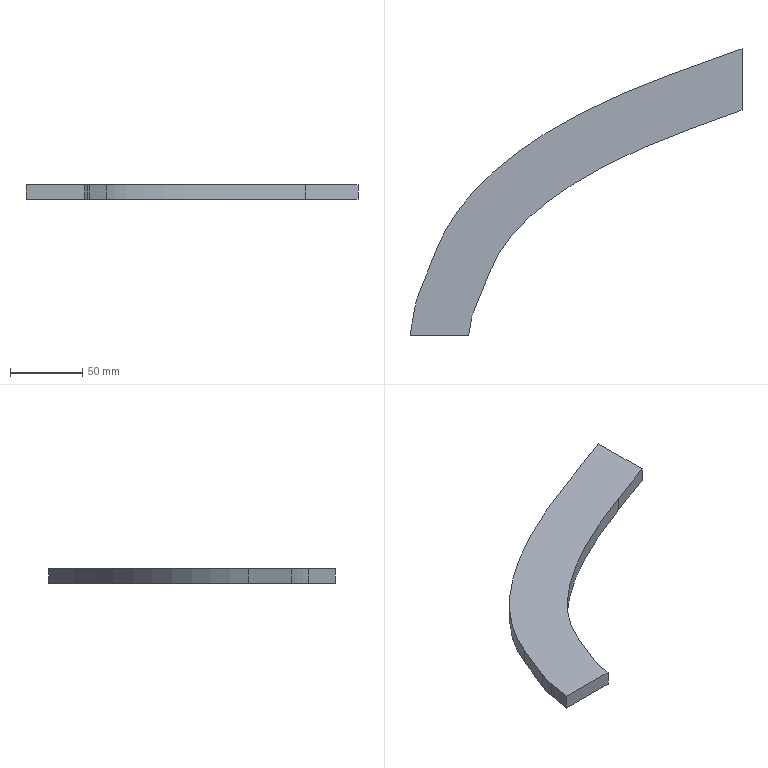Part | STEP file | 001-004-Feeding mechanism shaft entry channel plate | 1 solid | 14 faces | box 230 x 198.5 x 10 mm | volume 116591 mm3 | plane 10 | spline 2 | cylinder 2 | commonest cylinder face diameters 40 x1 120 x1
STEP:
#1=CARTESIAN_POINT('',(0.,0.,0.));
#2=DIRECTION('',(0.,0.,1.));
#3=DIRECTION('',(1.,0.,0.));
#4=AXIS2_PLACEMENT_3D('',#1,#2,#3);
#5=CARTESIAN_POINT('',(193.681,142.714,0.));
#6=VERTEX_POINT('',#5);
#7=CARTESIAN_POINT('',(55.723,45.016,0.));
#8=VERTEX_POINT('',#7);
#9=CARTESIAN_POINT('',(193.681,142.714,0.));
#10=CARTESIAN_POINT('',(192.392,142.245,0.));
#11=CARTESIAN_POINT('',(189.806,141.294,0.));
#12=CARTESIAN_POINT('',(184.734,139.392,0.));
#13=CARTESIAN_POINT('',(178.522,136.99,0.));
#14=CARTESIAN_POINT('',(171.29,134.077,0.));
#15=CARTESIAN_POINT('',(161.939,130.153,0.));
#16=CARTESIAN_POINT('',(150.802,125.175,0.));
#17=CARTESIAN_POINT('',(138.324,119.1,0.));
#18=CARTESIAN_POINT('',(126.736,112.936,0.));
#19=CARTESIAN_POINT('',(112.474,104.623,0.));
#20=CARTESIAN_POINT('',(96.878,94.103,0.));
#21=CARTESIAN_POINT('',(81.696,81.455,0.));
#22=CARTESIAN_POINT('',(71.878,71.064,0.));
#23=CARTESIAN_POINT('',(65.588,62.913,0.));
#24=CARTESIAN_POINT('',(61.605,56.882,0.));
#25=CARTESIAN_POINT('',(58.854,51.921,0.));
#26=CARTESIAN_POINT('',(56.963,47.967,0.));
#27=CARTESIAN_POINT('',(56.125,46.01,0.));
#28=CARTESIAN_POINT('',(55.723,45.016,0.));
#29=B_SPLINE_CURVE_WITH_KNOTS('',3,(#9,#10,#11,#12,#13,#14,#15,#16,#17,#18,#19,#20,#21,#22,#23,#24,#25,#26,#27,#28),.UNSPECIFIED.,.F.,.F.,(4,1,1,1,1,1,1,1,1,1,1,1,1,1,1,1,1,4),(0.,0.01562,0.03125,0.0625,0.09375,0.125,0.1875,0.25,0.3125,0.375,0.5,0.625,0.75,0.8125,0.875,0.9375,0.9688,1.),.UNSPECIFIED.);
#30=CARTESIAN_POINT('',(193.681,142.714,10.));
#31=CARTESIAN_POINT('',(193.681,142.714,0.));
#32=CARTESIAN_POINT('',(192.392,142.245,10.));
#33=CARTESIAN_POINT('',(192.392,142.245,0.));
#34=CARTESIAN_POINT('',(189.806,141.294,10.));
#35=CARTESIAN_POINT('',(189.806,141.294,0.));
#36=CARTESIAN_POINT('',(184.734,139.392,10.));
#37=CARTESIAN_POINT('',(184.734,139.392,0.));
#38=CARTESIAN_POINT('',(178.522,136.99,10.));
#39=CARTESIAN_POINT('',(178.522,136.99,0.));
#40=CARTESIAN_POINT('',(171.29,134.077,10.));
#41=CARTESIAN_POINT('',(171.29,134.077,0.));
#42=CARTESIAN_POINT('',(161.939,130.153,10.));
#43=CARTESIAN_POINT('',(161.939,130.153,0.));
#44=CARTESIAN_POINT('',(150.802,125.175,10.));
#45=CARTESIAN_POINT('',(150.802,125.175,0.));
#46=CARTESIAN_POINT('',(138.324,119.1,10.));
#47=CARTESIAN_POINT('',(138.324,119.1,0.));
#48=CARTESIAN_POINT('',(126.736,112.936,10.));
#49=CARTESIAN_POINT('',(126.736,112.936,0.));
#50=CARTESIAN_POINT('',(112.474,104.623,10.));
#51=CARTESIAN_POINT('',(112.474,104.623,0.));
#52=CARTESIAN_POINT('',(96.878,94.103,10.));
#53=CARTESIAN_POINT('',(96.878,94.103,0.));
#54=CARTESIAN_POINT('',(81.696,81.455,10.));
#55=CARTESIAN_POINT('',(81.696,81.455,0.));
#56=CARTESIAN_POINT('',(71.878,71.064,10.));
#57=CARTESIAN_POINT('',(71.878,71.064,0.));
#58=CARTESIAN_POINT('',(65.588,62.913,10.));
#59=CARTESIAN_POINT('',(65.588,62.913,0.));
#60=CARTESIAN_POINT('',(61.605,56.882,10.));
#61=CARTESIAN_POINT('',(61.605,56.882,0.));
#62=CARTESIAN_POINT('',(58.854,51.921,10.));
#63=CARTESIAN_POINT('',(58.854,51.921,0.));
#64=CARTESIAN_POINT('',(56.963,47.967,10.));
#65=CARTESIAN_POINT('',(56.963,47.967,0.));
#66=CARTESIAN_POINT('',(56.125,46.01,10.));
#67=CARTESIAN_POINT('',(56.125,46.01,0.));
#68=CARTESIAN_POINT('',(55.723,45.016,10.));
#69=CARTESIAN_POINT('',(55.723,45.016,0.));
#70=B_SPLINE_SURFACE_WITH_KNOTS('',3,1,((#30,#31),(#32,#33),(#34,#35),(#36,#37),(#38,#39),(#40,#41),(#42,#43),(#44,#45),(#46,#47),(#48,#49),(#50,#51),(#52,#53),(#54,#55),(#56,#57),(#58,#59),(#60,#61),(#62,#63),(#64,#65),(#66,#67),(#68,#69)),.UNSPECIFIED.,.F.,.F.,.F.,(4,1,1,1,1,1,1,1,1,1,1,1,1,1,1,1,1,4),(2,2),(0.,0.01562,0.03125,0.0625,0.09375,0.125,0.1875,0.25,0.3125,0.375,0.5,0.625,0.75,0.8125,0.875,0.9375,0.9688,1.),(0.,1.),.UNSPECIFIED.);
#71=CARTESIAN_POINT('',(0.,1.));
#72=DIRECTION('',(1.,0.));
#73=VECTOR('',#72,1.);
#74=LINE('',#71,#73);
#75=(GEOMETRIC_REPRESENTATION_CONTEXT(2)PARAMETRIC_REPRESENTATION_CONTEXT()REPRESENTATION_CONTEXT('',''));
#76=DEFINITIONAL_REPRESENTATION('',(#74),#75);
#77=PCURVE('',#70,#76);
#78=CARTESIAN_POINT('',(0.,0.,0.));
#79=DIRECTION('',(0.,0.,1.));
#80=DIRECTION('',(1.,0.,0.));
#81=AXIS2_PLACEMENT_3D('',#78,#79,#80);
#82=PLANE('',#81);
#83=CARTESIAN_POINT('',(193.681,142.714));
#84=CARTESIAN_POINT('',(192.392,142.245));
#85=CARTESIAN_POINT('',(189.806,141.294));
#86=CARTESIAN_POINT('',(184.734,139.392));
#87=CARTESIAN_POINT('',(178.522,136.99));
#88=CARTESIAN_POINT('',(171.29,134.077));
#89=CARTESIAN_POINT('',(161.939,130.153));
#90=CARTESIAN_POINT('',(150.802,125.175));
#91=CARTESIAN_POINT('',(138.324,119.1));
#92=CARTESIAN_POINT('',(126.736,112.936));
#93=CARTESIAN_POINT('',(112.474,104.623));
#94=CARTESIAN_POINT('',(96.878,94.103));
#95=CARTESIAN_POINT('',(81.696,81.455));
#96=CARTESIAN_POINT('',(71.878,71.064));
#97=CARTESIAN_POINT('',(65.588,62.913));
#98=CARTESIAN_POINT('',(61.605,56.882));
#99=CARTESIAN_POINT('',(58.854,51.921));
#100=CARTESIAN_POINT('',(56.963,47.967));
#101=CARTESIAN_POINT('',(56.125,46.01));
#102=CARTESIAN_POINT('',(55.723,45.016));
#103=B_SPLINE_CURVE_WITH_KNOTS('',3,(#83,#84,#85,#86,#87,#88,#89,#90,#91,#92,#93,#94,#95,#96,#97,#98,#99,#100,#101,#102),.UNSPECIFIED.,.F.,.F.,(4,1,1,1,1,1,1,1,1,1,1,1,1,1,1,1,1,4),(0.,0.01562,0.03125,0.0625,0.09375,0.125,0.1875,0.25,0.3125,0.375,0.5,0.625,0.75,0.8125,0.875,0.9375,0.9688,1.),.UNSPECIFIED.);
#104=(GEOMETRIC_REPRESENTATION_CONTEXT(2)PARAMETRIC_REPRESENTATION_CONTEXT()REPRESENTATION_CONTEXT('',''));
#105=DEFINITIONAL_REPRESENTATION('',(#103),#104);
#106=PCURVE('',#82,#105);
#107=SURFACE_CURVE('',#29,(#77,#106),.PCURVE_S1.);
#108=EDGE_CURVE('',#6,#8,#107,.T.);
#109=ORIENTED_EDGE('',*,*,#108,.F.);
#110=CARTESIAN_POINT('',(193.681,142.714,10.));
#111=VERTEX_POINT('',#110);
#112=CARTESIAN_POINT('',(193.681,142.714,10.));
#113=DIRECTION('',(0.,0.,-1.));
#114=VECTOR('',#113,1.);
#115=LINE('',#112,#114);
#116=CARTESIAN_POINT('',(0.,0.));
#117=CARTESIAN_POINT('',(0.,1.));
#118=B_SPLINE_CURVE_WITH_KNOTS('',1,(#116,#117),.UNSPECIFIED.,.F.,.F.,(2,2),(0.,10.),.PIECEWISE_BEZIER_KNOTS.);
#119=(GEOMETRIC_REPRESENTATION_CONTEXT(2)PARAMETRIC_REPRESENTATION_CONTEXT()REPRESENTATION_CONTEXT('',''));
#120=DEFINITIONAL_REPRESENTATION('',(#118),#119);
#121=PCURVE('',#70,#120);
#122=CARTESIAN_POINT('',(-23.211,63.772,10.));
#123=DIRECTION('',(0.342,-0.9397,0.));
#124=DIRECTION('',(0.9397,0.342,0.));
#125=AXIS2_PLACEMENT_3D('',#122,#123,#124);
#126=PLANE('',#125);
#127=CARTESIAN_POINT('',(230.811,0.));
#128=DIRECTION('',(0.,-1.));
#129=VECTOR('',#128,1.);
#130=LINE('',#127,#129);
#131=(GEOMETRIC_REPRESENTATION_CONTEXT(2)PARAMETRIC_REPRESENTATION_CONTEXT()REPRESENTATION_CONTEXT('',''));
#132=DEFINITIONAL_REPRESENTATION('',(#130),#131);
#133=PCURVE('',#126,#132);
#134=SURFACE_CURVE('',#115,(#121,#133),.PCURVE_S1.);
#135=EDGE_CURVE('',#111,#6,#134,.T.);
#136=ORIENTED_EDGE('',*,*,#135,.F.);
#137=CARTESIAN_POINT('',(55.723,45.016,10.));
#138=VERTEX_POINT('',#137);
#139=CARTESIAN_POINT('',(193.681,142.714,10.));
#140=CARTESIAN_POINT('',(192.392,142.245,10.));
#141=CARTESIAN_POINT('',(189.806,141.294,10.));
#142=CARTESIAN_POINT('',(184.734,139.392,10.));
#143=CARTESIAN_POINT('',(178.522,136.99,10.));
#144=CARTESIAN_POINT('',(171.29,134.077,10.));
#145=CARTESIAN_POINT('',(161.939,130.153,10.));
#146=CARTESIAN_POINT('',(150.802,125.175,10.));
#147=CARTESIAN_POINT('',(138.324,119.1,10.));
#148=CARTESIAN_POINT('',(126.736,112.936,10.));
#149=CARTESIAN_POINT('',(112.474,104.623,10.));
#150=CARTESIAN_POINT('',(96.878,94.103,10.));
#151=CARTESIAN_POINT('',(81.696,81.455,10.));
#152=CARTESIAN_POINT('',(71.878,71.064,10.));
#153=CARTESIAN_POINT('',(65.588,62.913,10.));
#154=CARTESIAN_POINT('',(61.605,56.882,10.));
#155=CARTESIAN_POINT('',(58.854,51.921,10.));
#156=CARTESIAN_POINT('',(56.963,47.967,10.));
#157=CARTESIAN_POINT('',(56.125,46.01,10.));
#158=CARTESIAN_POINT('',(55.723,45.016,10.));
#159=B_SPLINE_CURVE_WITH_KNOTS('',3,(#139,#140,#141,#142,#143,#144,#145,#146,#147,#148,#149,#150,#151,#152,#153,#154,#155,#156,#157,#158),.UNSPECIFIED.,.F.,.F.,(4,1,1,1,1,1,1,1,1,1,1,1,1,1,1,1,1,4),(0.,0.01562,0.03125,0.0625,0.09375,0.125,0.1875,0.25,0.3125,0.375,0.5,0.625,0.75,0.8125,0.875,0.9375,0.9688,1.),.UNSPECIFIED.);
#160=CARTESIAN_POINT('',(0.,0.));
#161=DIRECTION('',(1.,0.));
#162=VECTOR('',#161,1.);
#163=LINE('',#160,#162);
#164=(GEOMETRIC_REPRESENTATION_CONTEXT(2)PARAMETRIC_REPRESENTATION_CONTEXT()REPRESENTATION_CONTEXT('',''));
#165=DEFINITIONAL_REPRESENTATION('',(#163),#164);
#166=PCURVE('',#70,#165);
#167=CARTESIAN_POINT('',(0.,0.,10.));
#168=DIRECTION('',(0.,0.,1.));
#169=DIRECTION('',(1.,0.,0.));
#170=AXIS2_PLACEMENT_3D('',#167,#168,#169);
#171=PLANE('',#170);
#172=CARTESIAN_POINT('',(193.681,142.714));
#173=CARTESIAN_POINT('',(192.392,142.245));
#174=CARTESIAN_POINT('',(189.806,141.294));
#175=CARTESIAN_POINT('',(184.734,139.392));
#176=CARTESIAN_POINT('',(178.522,136.99));
#177=CARTESIAN_POINT('',(171.29,134.077));
#178=CARTESIAN_POINT('',(161.939,130.153));
#179=CARTESIAN_POINT('',(150.802,125.175));
#180=CARTESIAN_POINT('',(138.324,119.1));
#181=CARTESIAN_POINT('',(126.736,112.936));
#182=CARTESIAN_POINT('',(112.474,104.623));
#183=CARTESIAN_POINT('',(96.878,94.103));
#184=CARTESIAN_POINT('',(81.696,81.455));
#185=CARTESIAN_POINT('',(71.878,71.064));
#186=CARTESIAN_POINT('',(65.588,62.913));
#187=CARTESIAN_POINT('',(61.605,56.882));
#188=CARTESIAN_POINT('',(58.854,51.921));
#189=CARTESIAN_POINT('',(56.963,47.967));
#190=CARTESIAN_POINT('',(56.125,46.01));
#191=CARTESIAN_POINT('',(55.723,45.016));
#192=B_SPLINE_CURVE_WITH_KNOTS('',3,(#172,#173,#174,#175,#176,#177,#178,#179,#180,#181,#182,#183,#184,#185,#186,#187,#188,#189,#190,#191),.UNSPECIFIED.,.F.,.F.,(4,1,1,1,1,1,1,1,1,1,1,1,1,1,1,1,1,4),(0.,0.01562,0.03125,0.0625,0.09375,0.125,0.1875,0.25,0.3125,0.375,0.5,0.625,0.75,0.8125,0.875,0.9375,0.9688,1.),.UNSPECIFIED.);
#193=(GEOMETRIC_REPRESENTATION_CONTEXT(2)PARAMETRIC_REPRESENTATION_CONTEXT()REPRESENTATION_CONTEXT('',''));
#194=DEFINITIONAL_REPRESENTATION('',(#192),#193);
#195=PCURVE('',#171,#194);
#196=SURFACE_CURVE('',#159,(#166,#195),.PCURVE_S1.);
#197=EDGE_CURVE('',#111,#138,#196,.T.);
#198=ORIENTED_EDGE('',*,*,#197,.T.);
#199=CARTESIAN_POINT('',(55.723,45.016,10.));
#200=DIRECTION('',(0.,0.,-1.));
#201=VECTOR('',#200,1.);
#202=LINE('',#199,#201);
#203=CARTESIAN_POINT('',(1.,0.));
#204=CARTESIAN_POINT('',(1.,1.));
#205=B_SPLINE_CURVE_WITH_KNOTS('',1,(#203,#204),.UNSPECIFIED.,.F.,.F.,(2,2),(0.,10.),.PIECEWISE_BEZIER_KNOTS.);
#206=(GEOMETRIC_REPRESENTATION_CONTEXT(2)PARAMETRIC_REPRESENTATION_CONTEXT()REPRESENTATION_CONTEXT('',''));
#207=DEFINITIONAL_REPRESENTATION('',(#205),#206);
#208=PCURVE('',#70,#207);
#209=CARTESIAN_POINT('',(32.268,-13.037,10.));
#210=DIRECTION('',(-0.9272,0.3746,0.));
#211=DIRECTION('',(-0.3746,-0.9272,0.));
#212=AXIS2_PLACEMENT_3D('',#209,#210,#211);
#213=PLANE('',#212);
#214=CARTESIAN_POINT('',(-62.612,0.));
#215=DIRECTION('',(0.,-1.));
#216=VECTOR('',#215,1.);
#217=LINE('',#214,#216);
#218=(GEOMETRIC_REPRESENTATION_CONTEXT(2)PARAMETRIC_REPRESENTATION_CONTEXT()REPRESENTATION_CONTEXT('',''));
#219=DEFINITIONAL_REPRESENTATION('',(#217),#218);
#220=PCURVE('',#213,#219);
#221=SURFACE_CURVE('',#202,(#208,#220),.PCURVE_S1.);
#222=EDGE_CURVE('',#138,#8,#221,.T.);
#223=ORIENTED_EDGE('',*,*,#222,.T.);
#224=EDGE_LOOP('',(#109,#136,#198,#223));
#225=FACE_BOUND('',#224,.T.);
#226=ADVANCED_FACE('',(#225),#70,.T.);
#227=CARTESIAN_POINT('',(230.,155.933,0.));
#228=VERTEX_POINT('',#227);
#229=CARTESIAN_POINT('',(-23.211,63.772,0.));
#230=DIRECTION('',(-0.9397,-0.342,0.));
#231=VECTOR('',#230,1.);
#232=LINE('',#229,#231);
#233=CARTESIAN_POINT('',(0.,-10.));
#234=DIRECTION('',(-1.,0.));
#235=VECTOR('',#234,1.);
#236=LINE('',#233,#235);
#237=(GEOMETRIC_REPRESENTATION_CONTEXT(2)PARAMETRIC_REPRESENTATION_CONTEXT()REPRESENTATION_CONTEXT('',''));
#238=DEFINITIONAL_REPRESENTATION('',(#236),#237);
#239=PCURVE('',#126,#238);
#240=CARTESIAN_POINT('',(-23.211,63.772));
#241=DIRECTION('',(-0.9397,-0.342));
#242=VECTOR('',#241,1.);
#243=LINE('',#240,#242);
#244=(GEOMETRIC_REPRESENTATION_CONTEXT(2)PARAMETRIC_REPRESENTATION_CONTEXT()REPRESENTATION_CONTEXT('',''));
#245=DEFINITIONAL_REPRESENTATION('',(#243),#244);
#246=PCURVE('',#82,#245);
#247=SURFACE_CURVE('',#232,(#239,#246),.PCURVE_S1.);
#248=EDGE_CURVE('',#228,#6,#247,.T.);
#249=ORIENTED_EDGE('',*,*,#248,.F.);
#250=CARTESIAN_POINT('',(230.,155.933,10.));
#251=VERTEX_POINT('',#250);
#252=CARTESIAN_POINT('',(230.,155.933,10.));
#253=DIRECTION('',(0.,0.,-1.));
#254=VECTOR('',#253,1.);
#255=LINE('',#252,#254);
#256=CARTESIAN_POINT('',(269.461,0.));
#257=DIRECTION('',(0.,-1.));
#258=VECTOR('',#257,1.);
#259=LINE('',#256,#258);
#260=(GEOMETRIC_REPRESENTATION_CONTEXT(2)PARAMETRIC_REPRESENTATION_CONTEXT()REPRESENTATION_CONTEXT('',''));
#261=DEFINITIONAL_REPRESENTATION('',(#259),#260);
#262=PCURVE('',#126,#261);
#263=CARTESIAN_POINT('',(230.,0.,10.));
#264=DIRECTION('',(-1.,0.,0.));
#265=DIRECTION('',(0.,0.,1.));
#266=AXIS2_PLACEMENT_3D('',#263,#264,#265);
#267=PLANE('',#266);
#268=CARTESIAN_POINT('',(0.,155.933));
#269=DIRECTION('',(-1.,0.));
#270=VECTOR('',#269,1.);
#271=LINE('',#268,#270);
#272=(GEOMETRIC_REPRESENTATION_CONTEXT(2)PARAMETRIC_REPRESENTATION_CONTEXT()REPRESENTATION_CONTEXT('',''));
#273=DEFINITIONAL_REPRESENTATION('',(#271),#272);
#274=PCURVE('',#267,#273);
#275=SURFACE_CURVE('',#255,(#262,#274),.PCURVE_S1.);
#276=EDGE_CURVE('',#251,#228,#275,.T.);
#277=ORIENTED_EDGE('',*,*,#276,.F.);
#278=CARTESIAN_POINT('',(-23.211,63.772,10.));
#279=DIRECTION('',(-0.9397,-0.342,0.));
#280=VECTOR('',#279,1.);
#281=LINE('',#278,#280);
#282=CARTESIAN_POINT('',(0.,0.));
#283=DIRECTION('',(-1.,0.));
#284=VECTOR('',#283,1.);
#285=LINE('',#282,#284);
#286=(GEOMETRIC_REPRESENTATION_CONTEXT(2)PARAMETRIC_REPRESENTATION_CONTEXT()REPRESENTATION_CONTEXT('',''));
#287=DEFINITIONAL_REPRESENTATION('',(#285),#286);
#288=PCURVE('',#126,#287);
#289=CARTESIAN_POINT('',(-23.211,63.772));
#290=DIRECTION('',(-0.9397,-0.342));
#291=VECTOR('',#290,1.);
#292=LINE('',#289,#291);
#293=(GEOMETRIC_REPRESENTATION_CONTEXT(2)PARAMETRIC_REPRESENTATION_CONTEXT()REPRESENTATION_CONTEXT('',''));
#294=DEFINITIONAL_REPRESENTATION('',(#292),#293);
#295=PCURVE('',#171,#294);
#296=SURFACE_CURVE('',#281,(#288,#295),.PCURVE_S1.);
#297=EDGE_CURVE('',#251,#111,#296,.T.);
#298=ORIENTED_EDGE('',*,*,#297,.T.);
#299=ORIENTED_EDGE('',*,*,#135,.T.);
#300=EDGE_LOOP('',(#249,#277,#298,#299));
#301=FACE_BOUND('',#300,.T.);
#302=ADVANCED_FACE('',(#301),#126,.T.);
#303=CARTESIAN_POINT('',(230.,198.5,0.));
#304=VERTEX_POINT('',#303);
#305=CARTESIAN_POINT('',(230.,0.,0.));
#306=DIRECTION('',(0.,1.,0.));
#307=VECTOR('',#306,1.);
#308=LINE('',#305,#307);
#309=CARTESIAN_POINT('',(-10.,0.));
#310=DIRECTION('',(0.,1.));
#311=VECTOR('',#310,1.);
#312=LINE('',#309,#311);
#313=(GEOMETRIC_REPRESENTATION_CONTEXT(2)PARAMETRIC_REPRESENTATION_CONTEXT()REPRESENTATION_CONTEXT('',''));
#314=DEFINITIONAL_REPRESENTATION('',(#312),#313);
#315=PCURVE('',#267,#314);
#316=CARTESIAN_POINT('',(230.,0.));
#317=DIRECTION('',(0.,1.));
#318=VECTOR('',#317,1.);
#319=LINE('',#316,#318);
#320=(GEOMETRIC_REPRESENTATION_CONTEXT(2)PARAMETRIC_REPRESENTATION_CONTEXT()REPRESENTATION_CONTEXT('',''));
#321=DEFINITIONAL_REPRESENTATION('',(#319),#320);
#322=PCURVE('',#82,#321);
#323=SURFACE_CURVE('',#308,(#315,#322),.PCURVE_S1.);
#324=EDGE_CURVE('',#228,#304,#323,.T.);
#325=ORIENTED_EDGE('',*,*,#324,.T.);
#326=CARTESIAN_POINT('',(230.,198.5,10.));
#327=VERTEX_POINT('',#326);
#328=CARTESIAN_POINT('',(230.,198.5,10.));
#329=DIRECTION('',(0.,0.,-1.));
#330=VECTOR('',#329,1.);
#331=LINE('',#328,#330);
#332=CARTESIAN_POINT('',(0.,198.5));
#333=DIRECTION('',(-1.,0.));
#334=VECTOR('',#333,1.);
#335=LINE('',#332,#334);
#336=(GEOMETRIC_REPRESENTATION_CONTEXT(2)PARAMETRIC_REPRESENTATION_CONTEXT()REPRESENTATION_CONTEXT('',''));
#337=DEFINITIONAL_REPRESENTATION('',(#335),#336);
#338=PCURVE('',#267,#337);
#339=CARTESIAN_POINT('',(-36.892,101.359,10.));
#340=DIRECTION('',(0.342,-0.9397,0.));
#341=DIRECTION('',(0.9397,0.342,0.));
#342=AXIS2_PLACEMENT_3D('',#339,#340,#341);
#343=PLANE('',#342);
#344=CARTESIAN_POINT('',(284.02,0.));
#345=DIRECTION('',(0.,-1.));
#346=VECTOR('',#345,1.);
#347=LINE('',#344,#346);
#348=(GEOMETRIC_REPRESENTATION_CONTEXT(2)PARAMETRIC_REPRESENTATION_CONTEXT()REPRESENTATION_CONTEXT('',''));
#349=DEFINITIONAL_REPRESENTATION('',(#347),#348);
#350=PCURVE('',#343,#349);
#351=SURFACE_CURVE('',#331,(#338,#350),.PCURVE_S1.);
#352=EDGE_CURVE('',#327,#304,#351,.T.);
#353=ORIENTED_EDGE('',*,*,#352,.F.);
#354=CARTESIAN_POINT('',(230.,0.,10.));
#355=DIRECTION('',(0.,1.,0.));
#356=VECTOR('',#355,1.);
#357=LINE('',#354,#356);
#358=CARTESIAN_POINT('',(0.,0.));
#359=DIRECTION('',(0.,1.));
#360=VECTOR('',#359,1.);
#361=LINE('',#358,#360);
#362=(GEOMETRIC_REPRESENTATION_CONTEXT(2)PARAMETRIC_REPRESENTATION_CONTEXT()REPRESENTATION_CONTEXT('',''));
#363=DEFINITIONAL_REPRESENTATION('',(#361),#362);
#364=PCURVE('',#267,#363);
#365=CARTESIAN_POINT('',(230.,0.));
#366=DIRECTION('',(0.,1.));
#367=VECTOR('',#366,1.);
#368=LINE('',#365,#367);
#369=(GEOMETRIC_REPRESENTATION_CONTEXT(2)PARAMETRIC_REPRESENTATION_CONTEXT()REPRESENTATION_CONTEXT('',''));
#370=DEFINITIONAL_REPRESENTATION('',(#368),#369);
#371=PCURVE('',#171,#370);
#372=SURFACE_CURVE('',#357,(#364,#371),.PCURVE_S1.);
#373=EDGE_CURVE('',#251,#327,#372,.T.);
#374=ORIENTED_EDGE('',*,*,#373,.F.);
#375=ORIENTED_EDGE('',*,*,#276,.T.);
#376=EDGE_LOOP('',(#325,#353,#374,#375));
#377=FACE_BOUND('',#376,.T.);
#378=ADVANCED_FACE('',(#377),#267,.F.);
#379=CARTESIAN_POINT('',(180.,180.301,0.));
#380=VERTEX_POINT('',#379);
#381=CARTESIAN_POINT('',(-36.892,101.359,0.));
#382=DIRECTION('',(-0.9397,-0.342,0.));
#383=VECTOR('',#382,1.);
#384=LINE('',#381,#383);
#385=CARTESIAN_POINT('',(0.,-10.));
#386=DIRECTION('',(-1.,0.));
#387=VECTOR('',#386,1.);
#388=LINE('',#385,#387);
#389=(GEOMETRIC_REPRESENTATION_CONTEXT(2)PARAMETRIC_REPRESENTATION_CONTEXT()REPRESENTATION_CONTEXT('',''));
#390=DEFINITIONAL_REPRESENTATION('',(#388),#389);
#391=PCURVE('',#343,#390);
#392=CARTESIAN_POINT('',(-36.892,101.359));
#393=DIRECTION('',(-0.9397,-0.342));
#394=VECTOR('',#393,1.);
#395=LINE('',#392,#394);
#396=(GEOMETRIC_REPRESENTATION_CONTEXT(2)PARAMETRIC_REPRESENTATION_CONTEXT()REPRESENTATION_CONTEXT('',''));
#397=DEFINITIONAL_REPRESENTATION('',(#395),#396);
#398=PCURVE('',#82,#397);
#399=SURFACE_CURVE('',#384,(#391,#398),.PCURVE_S1.);
#400=EDGE_CURVE('',#304,#380,#399,.T.);
#401=ORIENTED_EDGE('',*,*,#400,.T.);
#402=CARTESIAN_POINT('',(180.,180.301,10.));
#403=VERTEX_POINT('',#402);
#404=CARTESIAN_POINT('',(180.,180.301,10.));
#405=DIRECTION('',(0.,0.,-1.));
#406=VECTOR('',#405,1.);
#407=LINE('',#404,#406);
#408=CARTESIAN_POINT('',(230.811,0.));
#409=DIRECTION('',(0.,-1.));
#410=VECTOR('',#409,1.);
#411=LINE('',#408,#410);
#412=(GEOMETRIC_REPRESENTATION_CONTEXT(2)PARAMETRIC_REPRESENTATION_CONTEXT()REPRESENTATION_CONTEXT('',''));
#413=DEFINITIONAL_REPRESENTATION('',(#411),#412);
#414=PCURVE('',#343,#413);
#415=CARTESIAN_POINT('',(180.,180.301,10.));
#416=CARTESIAN_POINT('',(180.,180.301,0.));
#417=CARTESIAN_POINT('',(47.8,132.185,10.));
#418=CARTESIAN_POINT('',(47.8,132.185,0.));
#419=CARTESIAN_POINT('',(18.636,60.,10.));
#420=CARTESIAN_POINT('',(18.636,60.,0.));
#421=B_SPLINE_SURFACE_WITH_KNOTS('',2,1,((#415,#416),(#417,#418),(#419,#420)),.UNSPECIFIED.,.F.,.F.,.F.,(3,3),(2,2),(0.,1.),(0.,1.),.PIECEWISE_BEZIER_KNOTS.);
#422=CARTESIAN_POINT('',(0.,0.));
#423=CARTESIAN_POINT('',(0.,1.));
#424=B_SPLINE_CURVE_WITH_KNOTS('',1,(#422,#423),.UNSPECIFIED.,.F.,.F.,(2,2),(0.,10.),.PIECEWISE_BEZIER_KNOTS.);
#425=(GEOMETRIC_REPRESENTATION_CONTEXT(2)PARAMETRIC_REPRESENTATION_CONTEXT()REPRESENTATION_CONTEXT('',''));
#426=DEFINITIONAL_REPRESENTATION('',(#424),#425);
#427=PCURVE('',#421,#426);
#428=SURFACE_CURVE('',#407,(#414,#427),.PCURVE_S1.);
#429=EDGE_CURVE('',#403,#380,#428,.T.);
#430=ORIENTED_EDGE('',*,*,#429,.F.);
#431=CARTESIAN_POINT('',(-36.892,101.359,10.));
#432=DIRECTION('',(-0.9397,-0.342,0.));
#433=VECTOR('',#432,1.);
#434=LINE('',#431,#433);
#435=CARTESIAN_POINT('',(0.,0.));
#436=DIRECTION('',(-1.,0.));
#437=VECTOR('',#436,1.);
#438=LINE('',#435,#437);
#439=(GEOMETRIC_REPRESENTATION_CONTEXT(2)PARAMETRIC_REPRESENTATION_CONTEXT()REPRESENTATION_CONTEXT('',''));
#440=DEFINITIONAL_REPRESENTATION('',(#438),#439);
#441=PCURVE('',#343,#440);
#442=CARTESIAN_POINT('',(-36.892,101.359));
#443=DIRECTION('',(-0.9397,-0.342));
#444=VECTOR('',#443,1.);
#445=LINE('',#442,#444);
#446=(GEOMETRIC_REPRESENTATION_CONTEXT(2)PARAMETRIC_REPRESENTATION_CONTEXT()REPRESENTATION_CONTEXT('',''));
#447=DEFINITIONAL_REPRESENTATION('',(#445),#446);
#448=PCURVE('',#171,#447);
#449=SURFACE_CURVE('',#434,(#441,#448),.PCURVE_S1.);
#450=EDGE_CURVE('',#327,#403,#449,.T.);
#451=ORIENTED_EDGE('',*,*,#450,.F.);
#452=ORIENTED_EDGE('',*,*,#352,.T.);
#453=EDGE_LOOP('',(#401,#430,#451,#452));
#454=FACE_BOUND('',#453,.T.);
#455=ADVANCED_FACE('',(#454),#343,.F.);
#456=ORIENTED_EDGE('',*,*,#429,.F.);
#457=CARTESIAN_POINT('',(18.636,60.,10.));
#458=VERTEX_POINT('',#457);
#459=CARTESIAN_POINT('',(180.,180.301,10.));
#460=CARTESIAN_POINT('',(47.8,132.185,10.));
#461=CARTESIAN_POINT('',(18.636,60.,10.));
#462=B_SPLINE_CURVE_WITH_KNOTS('',2,(#459,#460,#461),.UNSPECIFIED.,.F.,.F.,(3,3),(0.,1.),.PIECEWISE_BEZIER_KNOTS.);
#463=CARTESIAN_POINT('',(0.,0.));
#464=DIRECTION('',(1.,0.));
#465=VECTOR('',#464,1.);
#466=LINE('',#463,#465);
#467=(GEOMETRIC_REPRESENTATION_CONTEXT(2)PARAMETRIC_REPRESENTATION_CONTEXT()REPRESENTATION_CONTEXT('',''));
#468=DEFINITIONAL_REPRESENTATION('',(#466),#467);
#469=PCURVE('',#421,#468);
#470=CARTESIAN_POINT('',(180.,180.301));
#471=CARTESIAN_POINT('',(47.8,132.185));
#472=CARTESIAN_POINT('',(18.636,60.));
#473=B_SPLINE_CURVE_WITH_KNOTS('',2,(#470,#471,#472),.UNSPECIFIED.,.F.,.F.,(3,3),(0.,1.),.PIECEWISE_BEZIER_KNOTS.);
#474=(GEOMETRIC_REPRESENTATION_CONTEXT(2)PARAMETRIC_REPRESENTATION_CONTEXT()REPRESENTATION_CONTEXT('',''));
#475=DEFINITIONAL_REPRESENTATION('',(#473),#474);
#476=PCURVE('',#171,#475);
#477=SURFACE_CURVE('',#462,(#469,#476),.PCURVE_S1.);
#478=EDGE_CURVE('',#403,#458,#477,.T.);
#479=ORIENTED_EDGE('',*,*,#478,.T.);
#480=CARTESIAN_POINT('',(18.636,60.,0.));
#481=VERTEX_POINT('',#480);
#482=CARTESIAN_POINT('',(18.636,60.,10.));
#483=DIRECTION('',(0.,0.,-1.));
#484=VECTOR('',#483,1.);
#485=LINE('',#482,#484);
#486=CARTESIAN_POINT('',(1.,0.));
#487=CARTESIAN_POINT('',(1.,1.));
#488=B_SPLINE_CURVE_WITH_KNOTS('',1,(#486,#487),.UNSPECIFIED.,.F.,.F.,(2,2),(0.,10.),.PIECEWISE_BEZIER_KNOTS.);
#489=(GEOMETRIC_REPRESENTATION_CONTEXT(2)PARAMETRIC_REPRESENTATION_CONTEXT()REPRESENTATION_CONTEXT('',''));
#490=DEFINITIONAL_REPRESENTATION('',(#488),#489);
#491=PCURVE('',#421,#490);
#492=CARTESIAN_POINT('',(-4.819,1.947,10.));
#493=DIRECTION('',(-0.9272,0.3746,0.));
#494=DIRECTION('',(-0.3746,-0.9272,0.));
#495=AXIS2_PLACEMENT_3D('',#492,#493,#494);
#496=PLANE('',#495);
#497=CARTESIAN_POINT('',(-62.612,0.));
#498=DIRECTION('',(0.,-1.));
#499=VECTOR('',#498,1.);
#500=LINE('',#497,#499);
#501=(GEOMETRIC_REPRESENTATION_CONTEXT(2)PARAMETRIC_REPRESENTATION_CONTEXT()REPRESENTATION_CONTEXT('',''));
#502=DEFINITIONAL_REPRESENTATION('',(#500),#501);
#503=PCURVE('',#496,#502);
#504=SURFACE_CURVE('',#485,(#491,#503),.PCURVE_S1.);
#505=EDGE_CURVE('',#458,#481,#504,.T.);
#506=ORIENTED_EDGE('',*,*,#505,.T.);
#507=CARTESIAN_POINT('',(180.,180.301,0.));
#508=CARTESIAN_POINT('',(47.8,132.185,0.));
#509=CARTESIAN_POINT('',(18.636,60.,0.));
#510=B_SPLINE_CURVE_WITH_KNOTS('',2,(#507,#508,#509),.UNSPECIFIED.,.F.,.F.,(3,3),(0.,1.),.PIECEWISE_BEZIER_KNOTS.);
#511=CARTESIAN_POINT('',(0.,1.));
#512=DIRECTION('',(1.,0.));
#513=VECTOR('',#512,1.);
#514=LINE('',#511,#513);
#515=(GEOMETRIC_REPRESENTATION_CONTEXT(2)PARAMETRIC_REPRESENTATION_CONTEXT()REPRESENTATION_CONTEXT('',''));
#516=DEFINITIONAL_REPRESENTATION('',(#514),#515);
#517=PCURVE('',#421,#516);
#518=CARTESIAN_POINT('',(180.,180.301));
#519=CARTESIAN_POINT('',(47.8,132.185));
#520=CARTESIAN_POINT('',(18.636,60.));
#521=B_SPLINE_CURVE_WITH_KNOTS('',2,(#518,#519,#520),.UNSPECIFIED.,.F.,.F.,(3,3),(0.,1.),.PIECEWISE_BEZIER_KNOTS.);
#522=(GEOMETRIC_REPRESENTATION_CONTEXT(2)PARAMETRIC_REPRESENTATION_CONTEXT()REPRESENTATION_CONTEXT('',''));
#523=DEFINITIONAL_REPRESENTATION('',(#521),#522);
#524=PCURVE('',#82,#523);
#525=SURFACE_CURVE('',#510,(#517,#524),.PCURVE_S1.);
#526=EDGE_CURVE('',#380,#481,#525,.T.);
#527=ORIENTED_EDGE('',*,*,#526,.F.);
#528=EDGE_LOOP('',(#456,#479,#506,#527));
#529=FACE_BOUND('',#528,.F.);
#530=ADVANCED_FACE('',(#529),#421,.F.);
#531=CARTESIAN_POINT('',(6.704,30.467,0.));
#532=VERTEX_POINT('',#531);
#533=CARTESIAN_POINT('',(-4.819,1.947,0.));
#534=DIRECTION('',(0.3746,0.9272,0.));
#535=VECTOR('',#534,1.);
#536=LINE('',#533,#535);
#537=CARTESIAN_POINT('',(0.,-10.));
#538=DIRECTION('',(-1.,0.));
#539=VECTOR('',#538,1.);
#540=LINE('',#537,#539);
#541=(GEOMETRIC_REPRESENTATION_CONTEXT(2)PARAMETRIC_REPRESENTATION_CONTEXT()REPRESENTATION_CONTEXT('',''));
#542=DEFINITIONAL_REPRESENTATION('',(#540),#541);
#543=PCURVE('',#496,#542);
#544=CARTESIAN_POINT('',(-4.819,1.947));
#545=DIRECTION('',(0.3746,0.9272));
#546=VECTOR('',#545,1.);
#547=LINE('',#544,#546);
#548=(GEOMETRIC_REPRESENTATION_CONTEXT(2)PARAMETRIC_REPRESENTATION_CONTEXT()REPRESENTATION_CONTEXT('',''));
#549=DEFINITIONAL_REPRESENTATION('',(#547),#548);
#550=PCURVE('',#82,#549);
#551=SURFACE_CURVE('',#536,(#543,#550),.PCURVE_S1.);
#552=EDGE_CURVE('',#532,#481,#551,.T.);
#553=ORIENTED_EDGE('',*,*,#552,.F.);
#554=CARTESIAN_POINT('',(6.704,30.467,10.));
#555=VERTEX_POINT('',#554);
#556=CARTESIAN_POINT('',(6.704,30.467,10.));
#557=DIRECTION('',(0.,0.,-1.));
#558=VECTOR('',#557,1.);
#559=LINE('',#556,#558);
#560=CARTESIAN_POINT('',(-30.76,0.));
#561=DIRECTION('',(0.,-1.));
#562=VECTOR('',#561,1.);
#563=LINE('',#560,#562);
#564=(GEOMETRIC_REPRESENTATION_CONTEXT(2)PARAMETRIC_REPRESENTATION_CONTEXT()REPRESENTATION_CONTEXT('',''));
#565=DEFINITIONAL_REPRESENTATION('',(#563),#564);
#566=PCURVE('',#496,#565);
#567=CARTESIAN_POINT('',(62.335,7.991,10.));
#568=DIRECTION('',(0.,0.,-1.));
#569=DIRECTION('',(-1.,0.,0.));
#570=AXIS2_PLACEMENT_3D('',#567,#568,#569);
#571=CYLINDRICAL_SURFACE('',#570,60.);
#572=CARTESIAN_POINT('',(0.384,0.));
#573=DIRECTION('',(0.,1.));
#574=VECTOR('',#573,1.);
#575=LINE('',#572,#574);
#576=(GEOMETRIC_REPRESENTATION_CONTEXT(2)PARAMETRIC_REPRESENTATION_CONTEXT()REPRESENTATION_CONTEXT('',''));
#577=DEFINITIONAL_REPRESENTATION('',(#575),#576);
#578=PCURVE('',#571,#577);
#579=SURFACE_CURVE('',#559,(#566,#578),.PCURVE_S1.);
#580=EDGE_CURVE('',#555,#532,#579,.T.);
#581=ORIENTED_EDGE('',*,*,#580,.F.);
#582=CARTESIAN_POINT('',(-4.819,1.947,10.));
#583=DIRECTION('',(0.3746,0.9272,0.));
#584=VECTOR('',#583,1.);
#585=LINE('',#582,#584);
#586=CARTESIAN_POINT('',(0.,0.));
#587=DIRECTION('',(-1.,0.));
#588=VECTOR('',#587,1.);
#589=LINE('',#586,#588);
#590=(GEOMETRIC_REPRESENTATION_CONTEXT(2)PARAMETRIC_REPRESENTATION_CONTEXT()REPRESENTATION_CONTEXT('',''));
#591=DEFINITIONAL_REPRESENTATION('',(#589),#590);
#592=PCURVE('',#496,#591);
#593=CARTESIAN_POINT('',(-4.819,1.947));
#594=DIRECTION('',(0.3746,0.9272));
#595=VECTOR('',#594,1.);
#596=LINE('',#593,#595);
#597=(GEOMETRIC_REPRESENTATION_CONTEXT(2)PARAMETRIC_REPRESENTATION_CONTEXT()REPRESENTATION_CONTEXT('',''));
#598=DEFINITIONAL_REPRESENTATION('',(#596),#597);
#599=PCURVE('',#171,#598);
#600=SURFACE_CURVE('',#585,(#592,#599),.PCURVE_S1.);
#601=EDGE_CURVE('',#555,#458,#600,.T.);
#602=ORIENTED_EDGE('',*,*,#601,.T.);
#603=ORIENTED_EDGE('',*,*,#505,.T.);
#604=EDGE_LOOP('',(#553,#581,#602,#603));
#605=FACE_BOUND('',#604,.T.);
#606=ADVANCED_FACE('',(#605),#496,.T.);
#607=CARTESIAN_POINT('',(3.246,18.41,0.));
#608=VERTEX_POINT('',#607);
#609=CARTESIAN_POINT('',(62.335,7.991,0.));
#610=DIRECTION('',(0.,0.,1.));
#611=DIRECTION('',(1.,0.,0.));
#612=AXIS2_PLACEMENT_3D('',#609,#610,#611);
#613=CIRCLE('',#612,60.);
#614=CARTESIAN_POINT('',(3.142,10.));
#615=DIRECTION('',(-1.,0.));
#616=VECTOR('',#615,1.);
#617=LINE('',#614,#616);
#618=(GEOMETRIC_REPRESENTATION_CONTEXT(2)PARAMETRIC_REPRESENTATION_CONTEXT()REPRESENTATION_CONTEXT('',''));
#619=DEFINITIONAL_REPRESENTATION('',(#617),#618);
#620=PCURVE('',#571,#619);
#621=CARTESIAN_POINT('',(62.335,7.991));
#622=DIRECTION('',(1.,0.));
#623=AXIS2_PLACEMENT_2D('',#621,#622);
#624=CIRCLE('',#623,60.);
#625=(GEOMETRIC_REPRESENTATION_CONTEXT(2)PARAMETRIC_REPRESENTATION_CONTEXT()REPRESENTATION_CONTEXT('',''));
#626=DEFINITIONAL_REPRESENTATION('',(#624),#625);
#627=PCURVE('',#82,#626);
#628=SURFACE_CURVE('',#613,(#620,#627),.PCURVE_S1.);
#629=EDGE_CURVE('',#532,#608,#628,.T.);
#630=ORIENTED_EDGE('',*,*,#629,.T.);
#631=CARTESIAN_POINT('',(3.246,18.41,10.));
#632=VERTEX_POINT('',#631);
#633=CARTESIAN_POINT('',(3.246,18.41,10.));
#634=DIRECTION('',(0.,0.,-1.));
#635=VECTOR('',#634,1.);
#636=LINE('',#633,#635);
#637=CARTESIAN_POINT('',(0.1745,0.));
#638=DIRECTION('',(0.,1.));
#639=VECTOR('',#638,1.);
#640=LINE('',#637,#639);
#641=(GEOMETRIC_REPRESENTATION_CONTEXT(2)PARAMETRIC_REPRESENTATION_CONTEXT()REPRESENTATION_CONTEXT('',''));
#642=DEFINITIONAL_REPRESENTATION('',(#640),#641);
#643=PCURVE('',#571,#642);
#644=CARTESIAN_POINT('',(0.,0.,10.));
#645=DIRECTION('',(-0.9848,0.1736,0.));
#646=DIRECTION('',(-0.1736,-0.9848,0.));
#647=AXIS2_PLACEMENT_3D('',#644,#645,#646);
#648=PLANE('',#647);
#649=CARTESIAN_POINT('',(-18.694,0.));
#650=DIRECTION('',(0.,-1.));
#651=VECTOR('',#650,1.);
#652=LINE('',#649,#651);
#653=(GEOMETRIC_REPRESENTATION_CONTEXT(2)PARAMETRIC_REPRESENTATION_CONTEXT()REPRESENTATION_CONTEXT('',''));
#654=DEFINITIONAL_REPRESENTATION('',(#652),#653);
#655=PCURVE('',#648,#654);
#656=SURFACE_CURVE('',#636,(#643,#655),.PCURVE_S1.);
#657=EDGE_CURVE('',#632,#608,#656,.T.);
#658=ORIENTED_EDGE('',*,*,#657,.F.);
#659=CARTESIAN_POINT('',(62.335,7.991,10.));
#660=DIRECTION('',(0.,0.,1.));
#661=DIRECTION('',(1.,0.,0.));
#662=AXIS2_PLACEMENT_3D('',#659,#660,#661);
#663=CIRCLE('',#662,60.);
#664=CARTESIAN_POINT('',(3.142,0.));
#665=DIRECTION('',(-1.,0.));
#666=VECTOR('',#665,1.);
#667=LINE('',#664,#666);
#668=(GEOMETRIC_REPRESENTATION_CONTEXT(2)PARAMETRIC_REPRESENTATION_CONTEXT()REPRESENTATION_CONTEXT('',''));
#669=DEFINITIONAL_REPRESENTATION('',(#667),#668);
#670=PCURVE('',#571,#669);
#671=CARTESIAN_POINT('',(62.335,7.991));
#672=DIRECTION('',(1.,0.));
#673=AXIS2_PLACEMENT_2D('',#671,#672);
#674=CIRCLE('',#673,60.);
#675=(GEOMETRIC_REPRESENTATION_CONTEXT(2)PARAMETRIC_REPRESENTATION_CONTEXT()REPRESENTATION_CONTEXT('',''));
#676=DEFINITIONAL_REPRESENTATION('',(#674),#675);
#677=PCURVE('',#171,#676);
#678=SURFACE_CURVE('',#663,(#670,#677),.PCURVE_S1.);
#679=EDGE_CURVE('',#555,#632,#678,.T.);
#680=ORIENTED_EDGE('',*,*,#679,.F.);
#681=ORIENTED_EDGE('',*,*,#580,.T.);
#682=EDGE_LOOP('',(#630,#658,#680,#681));
#683=FACE_BOUND('',#682,.T.);
#684=ADVANCED_FACE('',(#683),#571,.T.);
#685=CARTESIAN_POINT('',(0.,0.,0.));
#686=VERTEX_POINT('',#685);
#687=CARTESIAN_POINT('',(0.,0.,0.));
#688=DIRECTION('',(0.1736,0.9848,0.));
#689=VECTOR('',#688,1.);
#690=LINE('',#687,#689);
#691=CARTESIAN_POINT('',(0.,-10.));
#692=DIRECTION('',(-1.,0.));
#693=VECTOR('',#692,1.);
#694=LINE('',#691,#693);
#695=(GEOMETRIC_REPRESENTATION_CONTEXT(2)PARAMETRIC_REPRESENTATION_CONTEXT()REPRESENTATION_CONTEXT('',''));
#696=DEFINITIONAL_REPRESENTATION('',(#694),#695);
#697=PCURVE('',#648,#696);
#698=CARTESIAN_POINT('',(0.,0.));
#699=DIRECTION('',(0.1736,0.9848));
#700=VECTOR('',#699,1.);
#701=LINE('',#698,#700);
#702=(GEOMETRIC_REPRESENTATION_CONTEXT(2)PARAMETRIC_REPRESENTATION_CONTEXT()REPRESENTATION_CONTEXT('',''));
#703=DEFINITIONAL_REPRESENTATION('',(#701),#702);
#704=PCURVE('',#82,#703);
#705=SURFACE_CURVE('',#690,(#697,#704),.PCURVE_S1.);
#706=EDGE_CURVE('',#686,#608,#705,.T.);
#707=ORIENTED_EDGE('',*,*,#706,.F.);
#708=CARTESIAN_POINT('',(0.,0.,10.));
#709=VERTEX_POINT('',#708);
#710=CARTESIAN_POINT('',(0.,0.,10.));
#711=DIRECTION('',(0.,0.,-1.));
#712=VECTOR('',#711,1.);
#713=LINE('',#710,#712);
#714=CARTESIAN_POINT('',(0.,0.));
#715=DIRECTION('',(0.,-1.));
#716=VECTOR('',#715,1.);
#717=LINE('',#714,#716);
#718=(GEOMETRIC_REPRESENTATION_CONTEXT(2)PARAMETRIC_REPRESENTATION_CONTEXT()REPRESENTATION_CONTEXT('',''));
#719=DEFINITIONAL_REPRESENTATION('',(#717),#718);
#720=PCURVE('',#648,#719);
#721=CARTESIAN_POINT('',(0.,0.,10.));
#722=DIRECTION('',(0.,1.,0.));
#723=DIRECTION('',(0.,0.,1.));
#724=AXIS2_PLACEMENT_3D('',#721,#722,#723);
#725=PLANE('',#724);
#726=CARTESIAN_POINT('',(0.,0.));
#727=DIRECTION('',(-1.,0.));
#728=VECTOR('',#727,1.);
#729=LINE('',#726,#728);
#730=(GEOMETRIC_REPRESENTATION_CONTEXT(2)PARAMETRIC_REPRESENTATION_CONTEXT()REPRESENTATION_CONTEXT('',''));
#731=DEFINITIONAL_REPRESENTATION('',(#729),#730);
#732=PCURVE('',#725,#731);
#733=SURFACE_CURVE('',#713,(#720,#732),.PCURVE_S1.);
#734=EDGE_CURVE('',#709,#686,#733,.T.);
#735=ORIENTED_EDGE('',*,*,#734,.F.);
#736=CARTESIAN_POINT('',(0.,0.,10.));
#737=DIRECTION('',(0.1736,0.9848,0.));
#738=VECTOR('',#737,1.);
#739=LINE('',#736,#738);
#740=CARTESIAN_POINT('',(0.,0.));
#741=DIRECTION('',(-1.,0.));
#742=VECTOR('',#741,1.);
#743=LINE('',#740,#742);
#744=(GEOMETRIC_REPRESENTATION_CONTEXT(2)PARAMETRIC_REPRESENTATION_CONTEXT()REPRESENTATION_CONTEXT('',''));
#745=DEFINITIONAL_REPRESENTATION('',(#743),#744);
#746=PCURVE('',#648,#745);
#747=CARTESIAN_POINT('',(0.,0.));
#748=DIRECTION('',(0.1736,0.9848));
#749=VECTOR('',#748,1.);
#750=LINE('',#747,#749);
#751=(GEOMETRIC_REPRESENTATION_CONTEXT(2)PARAMETRIC_REPRESENTATION_CONTEXT()REPRESENTATION_CONTEXT('',''));
#752=DEFINITIONAL_REPRESENTATION('',(#750),#751);
#753=PCURVE('',#171,#752);
#754=SURFACE_CURVE('',#739,(#746,#753),.PCURVE_S1.);
#755=EDGE_CURVE('',#709,#632,#754,.T.);
#756=ORIENTED_EDGE('',*,*,#755,.T.);
#757=ORIENTED_EDGE('',*,*,#657,.T.);
#758=EDGE_LOOP('',(#707,#735,#756,#757));
#759=FACE_BOUND('',#758,.T.);
#760=ADVANCED_FACE('',(#759),#648,.T.);
#761=CARTESIAN_POINT('',(40.617,0.,0.));
#762=VERTEX_POINT('',#761);
#763=CARTESIAN_POINT('',(0.,0.,0.));
#764=DIRECTION('',(1.,0.,0.));
#765=VECTOR('',#764,1.);
#766=LINE('',#763,#765);
#767=CARTESIAN_POINT('',(-10.,0.));
#768=DIRECTION('',(0.,1.));
#769=VECTOR('',#768,1.);
#770=LINE('',#767,#769);
#771=(GEOMETRIC_REPRESENTATION_CONTEXT(2)PARAMETRIC_REPRESENTATION_CONTEXT()REPRESENTATION_CONTEXT('',''));
#772=DEFINITIONAL_REPRESENTATION('',(#770),#771);
#773=PCURVE('',#725,#772);
#774=CARTESIAN_POINT('',(0.,0.));
#775=DIRECTION('',(1.,0.));
#776=VECTOR('',#775,1.);
#777=LINE('',#774,#776);
#778=(GEOMETRIC_REPRESENTATION_CONTEXT(2)PARAMETRIC_REPRESENTATION_CONTEXT()REPRESENTATION_CONTEXT('',''));
#779=DEFINITIONAL_REPRESENTATION('',(#777),#778);
#780=PCURVE('',#82,#779);
#781=SURFACE_CURVE('',#766,(#773,#780),.PCURVE_S1.);
#782=EDGE_CURVE('',#686,#762,#781,.T.);
#783=ORIENTED_EDGE('',*,*,#782,.T.);
#784=CARTESIAN_POINT('',(40.617,0.,10.));
#785=VERTEX_POINT('',#784);
#786=CARTESIAN_POINT('',(40.617,0.,10.));
#787=DIRECTION('',(0.,0.,-1.));
#788=VECTOR('',#787,1.);
#789=LINE('',#786,#788);
#790=CARTESIAN_POINT('',(0.,40.617));
#791=DIRECTION('',(-1.,0.));
#792=VECTOR('',#791,1.);
#793=LINE('',#790,#792);
#794=(GEOMETRIC_REPRESENTATION_CONTEXT(2)PARAMETRIC_REPRESENTATION_CONTEXT()REPRESENTATION_CONTEXT('',''));
#795=DEFINITIONAL_REPRESENTATION('',(#793),#794);
#796=PCURVE('',#725,#795);
#797=CARTESIAN_POINT('',(39.392,-6.946,10.));
#798=DIRECTION('',(-0.9848,0.1736,0.));
#799=DIRECTION('',(-0.1736,-0.9848,0.));
#800=AXIS2_PLACEMENT_3D('',#797,#798,#799);
#801=PLANE('',#800);
#802=CARTESIAN_POINT('',(-7.053,0.));
#803=DIRECTION('',(0.,-1.));
#804=VECTOR('',#803,1.);
#805=LINE('',#802,#804);
#806=(GEOMETRIC_REPRESENTATION_CONTEXT(2)PARAMETRIC_REPRESENTATION_CONTEXT()REPRESENTATION_CONTEXT('',''));
#807=DEFINITIONAL_REPRESENTATION('',(#805),#806);
#808=PCURVE('',#801,#807);
#809=SURFACE_CURVE('',#789,(#796,#808),.PCURVE_S1.);
#810=EDGE_CURVE('',#785,#762,#809,.T.);
#811=ORIENTED_EDGE('',*,*,#810,.F.);
#812=CARTESIAN_POINT('',(0.,0.,10.));
#813=DIRECTION('',(1.,0.,0.));
#814=VECTOR('',#813,1.);
#815=LINE('',#812,#814);
#816=CARTESIAN_POINT('',(0.,0.));
#817=DIRECTION('',(0.,1.));
#818=VECTOR('',#817,1.);
#819=LINE('',#816,#818);
#820=(GEOMETRIC_REPRESENTATION_CONTEXT(2)PARAMETRIC_REPRESENTATION_CONTEXT()REPRESENTATION_CONTEXT('',''));
#821=DEFINITIONAL_REPRESENTATION('',(#819),#820);
#822=PCURVE('',#725,#821);
#823=CARTESIAN_POINT('',(0.,0.));
#824=DIRECTION('',(1.,0.));
#825=VECTOR('',#824,1.);
#826=LINE('',#823,#825);
#827=(GEOMETRIC_REPRESENTATION_CONTEXT(2)PARAMETRIC_REPRESENTATION_CONTEXT()REPRESENTATION_CONTEXT('',''));
#828=DEFINITIONAL_REPRESENTATION('',(#826),#827);
#829=PCURVE('',#171,#828);
#830=SURFACE_CURVE('',#815,(#822,#829),.PCURVE_S1.);
#831=EDGE_CURVE('',#709,#785,#830,.T.);
#832=ORIENTED_EDGE('',*,*,#831,.F.);
#833=ORIENTED_EDGE('',*,*,#734,.T.);
#834=EDGE_LOOP('',(#783,#811,#832,#833));
#835=FACE_BOUND('',#834,.T.);
#836=ADVANCED_FACE('',(#835),#725,.F.);
#837=CARTESIAN_POINT('',(42.638,11.464,0.));
#838=VERTEX_POINT('',#837);
#839=CARTESIAN_POINT('',(39.392,-6.946,0.));
#840=DIRECTION('',(0.1736,0.9848,0.));
#841=VECTOR('',#840,1.);
#842=LINE('',#839,#841);
#843=CARTESIAN_POINT('',(0.,-10.));
#844=DIRECTION('',(-1.,0.));
#845=VECTOR('',#844,1.);
#846=LINE('',#843,#845);
#847=(GEOMETRIC_REPRESENTATION_CONTEXT(2)PARAMETRIC_REPRESENTATION_CONTEXT()REPRESENTATION_CONTEXT('',''));
#848=DEFINITIONAL_REPRESENTATION('',(#846),#847);
#849=PCURVE('',#801,#848);
#850=CARTESIAN_POINT('',(39.392,-6.946));
#851=DIRECTION('',(0.1736,0.9848));
#852=VECTOR('',#851,1.);
#853=LINE('',#850,#852);
#854=(GEOMETRIC_REPRESENTATION_CONTEXT(2)PARAMETRIC_REPRESENTATION_CONTEXT()REPRESENTATION_CONTEXT('',''));
#855=DEFINITIONAL_REPRESENTATION('',(#853),#854);
#856=PCURVE('',#82,#855);
#857=SURFACE_CURVE('',#842,(#849,#856),.PCURVE_S1.);
#858=EDGE_CURVE('',#762,#838,#857,.T.);
#859=ORIENTED_EDGE('',*,*,#858,.T.);
#860=CARTESIAN_POINT('',(42.638,11.464,10.));
#861=VERTEX_POINT('',#860);
#862=CARTESIAN_POINT('',(42.638,11.464,10.));
#863=DIRECTION('',(0.,0.,-1.));
#864=VECTOR('',#863,1.);
#865=LINE('',#862,#864);
#866=CARTESIAN_POINT('',(-18.694,0.));
#867=DIRECTION('',(0.,-1.));
#868=VECTOR('',#867,1.);
#869=LINE('',#866,#868);
#870=(GEOMETRIC_REPRESENTATION_CONTEXT(2)PARAMETRIC_REPRESENTATION_CONTEXT()REPRESENTATION_CONTEXT('',''));
#871=DEFINITIONAL_REPRESENTATION('',(#869),#870);
#872=PCURVE('',#801,#871);
#873=CARTESIAN_POINT('',(62.335,7.991,10.));
#874=DIRECTION('',(0.,0.,-1.));
#875=DIRECTION('',(-1.,0.,0.));
#876=AXIS2_PLACEMENT_3D('',#873,#874,#875);
#877=CYLINDRICAL_SURFACE('',#876,20.);
#878=CARTESIAN_POINT('',(0.1745,0.));
#879=DIRECTION('',(0.,1.));
#880=VECTOR('',#879,1.);
#881=LINE('',#878,#880);
#882=(GEOMETRIC_REPRESENTATION_CONTEXT(2)PARAMETRIC_REPRESENTATION_CONTEXT()REPRESENTATION_CONTEXT('',''));
#883=DEFINITIONAL_REPRESENTATION('',(#881),#882);
#884=PCURVE('',#877,#883);
#885=SURFACE_CURVE('',#865,(#872,#884),.PCURVE_S1.);
#886=EDGE_CURVE('',#861,#838,#885,.T.);
#887=ORIENTED_EDGE('',*,*,#886,.F.);
#888=CARTESIAN_POINT('',(39.392,-6.946,10.));
#889=DIRECTION('',(0.1736,0.9848,0.));
#890=VECTOR('',#889,1.);
#891=LINE('',#888,#890);
#892=CARTESIAN_POINT('',(0.,0.));
#893=DIRECTION('',(-1.,0.));
#894=VECTOR('',#893,1.);
#895=LINE('',#892,#894);
#896=(GEOMETRIC_REPRESENTATION_CONTEXT(2)PARAMETRIC_REPRESENTATION_CONTEXT()REPRESENTATION_CONTEXT('',''));
#897=DEFINITIONAL_REPRESENTATION('',(#895),#896);
#898=PCURVE('',#801,#897);
#899=CARTESIAN_POINT('',(39.392,-6.946));
#900=DIRECTION('',(0.1736,0.9848));
#901=VECTOR('',#900,1.);
#902=LINE('',#899,#901);
#903=(GEOMETRIC_REPRESENTATION_CONTEXT(2)PARAMETRIC_REPRESENTATION_CONTEXT()REPRESENTATION_CONTEXT('',''));
#904=DEFINITIONAL_REPRESENTATION('',(#902),#903);
#905=PCURVE('',#171,#904);
#906=SURFACE_CURVE('',#891,(#898,#905),.PCURVE_S1.);
#907=EDGE_CURVE('',#785,#861,#906,.T.);
#908=ORIENTED_EDGE('',*,*,#907,.F.);
#909=ORIENTED_EDGE('',*,*,#810,.T.);
#910=EDGE_LOOP('',(#859,#887,#908,#909));
#911=FACE_BOUND('',#910,.T.);
#912=ADVANCED_FACE('',(#911),#801,.F.);
#913=ORIENTED_EDGE('',*,*,#886,.F.);
#914=CARTESIAN_POINT('',(43.791,15.483,10.));
#915=VERTEX_POINT('',#914);
#916=CARTESIAN_POINT('',(62.335,7.991,10.));
#917=DIRECTION('',(0.,0.,1.));
#918=DIRECTION('',(1.,0.,0.));
#919=AXIS2_PLACEMENT_3D('',#916,#917,#918);
#920=CIRCLE('',#919,20.);
#921=CARTESIAN_POINT('',(3.142,0.));
#922=DIRECTION('',(-1.,0.));
#923=VECTOR('',#922,1.);
#924=LINE('',#921,#923);
#925=(GEOMETRIC_REPRESENTATION_CONTEXT(2)PARAMETRIC_REPRESENTATION_CONTEXT()REPRESENTATION_CONTEXT('',''));
#926=DEFINITIONAL_REPRESENTATION('',(#924),#925);
#927=PCURVE('',#877,#926);
#928=CARTESIAN_POINT('',(62.335,7.991));
#929=DIRECTION('',(1.,0.));
#930=AXIS2_PLACEMENT_2D('',#928,#929);
#931=CIRCLE('',#930,20.);
#932=(GEOMETRIC_REPRESENTATION_CONTEXT(2)PARAMETRIC_REPRESENTATION_CONTEXT()REPRESENTATION_CONTEXT('',''));
#933=DEFINITIONAL_REPRESENTATION('',(#931),#932);
#934=PCURVE('',#171,#933);
#935=SURFACE_CURVE('',#920,(#927,#934),.PCURVE_S1.);
#936=EDGE_CURVE('',#915,#861,#935,.T.);
#937=ORIENTED_EDGE('',*,*,#936,.F.);
#938=CARTESIAN_POINT('',(43.791,15.483,0.));
#939=VERTEX_POINT('',#938);
#940=CARTESIAN_POINT('',(43.791,15.483,10.));
#941=DIRECTION('',(0.,0.,-1.));
#942=VECTOR('',#941,1.);
#943=LINE('',#940,#942);
#944=CARTESIAN_POINT('',(0.384,0.));
#945=DIRECTION('',(0.,1.));
#946=VECTOR('',#945,1.);
#947=LINE('',#944,#946);
#948=(GEOMETRIC_REPRESENTATION_CONTEXT(2)PARAMETRIC_REPRESENTATION_CONTEXT()REPRESENTATION_CONTEXT('',''));
#949=DEFINITIONAL_REPRESENTATION('',(#947),#948);
#950=PCURVE('',#877,#949);
#951=CARTESIAN_POINT('',(-30.76,0.));
#952=DIRECTION('',(0.,-1.));
#953=VECTOR('',#952,1.);
#954=LINE('',#951,#953);
#955=(GEOMETRIC_REPRESENTATION_CONTEXT(2)PARAMETRIC_REPRESENTATION_CONTEXT()REPRESENTATION_CONTEXT('',''));
#956=DEFINITIONAL_REPRESENTATION('',(#954),#955);
#957=PCURVE('',#213,#956);
#958=SURFACE_CURVE('',#943,(#950,#957),.PCURVE_S1.);
#959=EDGE_CURVE('',#915,#939,#958,.T.);
#960=ORIENTED_EDGE('',*,*,#959,.T.);
#961=CARTESIAN_POINT('',(62.335,7.991,0.));
#962=DIRECTION('',(0.,0.,1.));
#963=DIRECTION('',(1.,0.,0.));
#964=AXIS2_PLACEMENT_3D('',#961,#962,#963);
#965=CIRCLE('',#964,20.);
#966=CARTESIAN_POINT('',(3.142,10.));
#967=DIRECTION('',(-1.,0.));
#968=VECTOR('',#967,1.);
#969=LINE('',#966,#968);
#970=(GEOMETRIC_REPRESENTATION_CONTEXT(2)PARAMETRIC_REPRESENTATION_CONTEXT()REPRESENTATION_CONTEXT('',''));
#971=DEFINITIONAL_REPRESENTATION('',(#969),#970);
#972=PCURVE('',#877,#971);
#973=CARTESIAN_POINT('',(62.335,7.991));
#974=DIRECTION('',(1.,0.));
#975=AXIS2_PLACEMENT_2D('',#973,#974);
#976=CIRCLE('',#975,20.);
#977=(GEOMETRIC_REPRESENTATION_CONTEXT(2)PARAMETRIC_REPRESENTATION_CONTEXT()REPRESENTATION_CONTEXT('',''));
#978=DEFINITIONAL_REPRESENTATION('',(#976),#977);
#979=PCURVE('',#82,#978);
#980=SURFACE_CURVE('',#965,(#972,#979),.PCURVE_S1.);
#981=EDGE_CURVE('',#939,#838,#980,.T.);
#982=ORIENTED_EDGE('',*,*,#981,.T.);
#983=EDGE_LOOP('',(#913,#937,#960,#982));
#984=FACE_BOUND('',#983,.F.);
#985=ADVANCED_FACE('',(#984),#877,.F.);
#986=CARTESIAN_POINT('',(32.268,-13.037,0.));
#987=DIRECTION('',(0.3746,0.9272,0.));
#988=VECTOR('',#987,1.);
#989=LINE('',#986,#988);
#990=CARTESIAN_POINT('',(0.,-10.));
#991=DIRECTION('',(-1.,0.));
#992=VECTOR('',#991,1.);
#993=LINE('',#990,#992);
#994=(GEOMETRIC_REPRESENTATION_CONTEXT(2)PARAMETRIC_REPRESENTATION_CONTEXT()REPRESENTATION_CONTEXT('',''));
#995=DEFINITIONAL_REPRESENTATION('',(#993),#994);
#996=PCURVE('',#213,#995);
#997=CARTESIAN_POINT('',(32.268,-13.037));
#998=DIRECTION('',(0.3746,0.9272));
#999=VECTOR('',#998,1.);
#1000=LINE('',#997,#999);
#1001=(GEOMETRIC_REPRESENTATION_CONTEXT(2)PARAMETRIC_REPRESENTATION_CONTEXT()REPRESENTATION_CONTEXT('',''));
#1002=DEFINITIONAL_REPRESENTATION('',(#1000),#1001);
#1003=PCURVE('',#82,#1002);
#1004=SURFACE_CURVE('',#989,(#996,#1003),.PCURVE_S1.);
#1005=EDGE_CURVE('',#939,#8,#1004,.T.);
#1006=ORIENTED_EDGE('',*,*,#1005,.T.);
#1007=ORIENTED_EDGE('',*,*,#222,.F.);
#1008=CARTESIAN_POINT('',(32.268,-13.037,10.));
#1009=DIRECTION('',(0.3746,0.9272,0.));
#1010=VECTOR('',#1009,1.);
#1011=LINE('',#1008,#1010);
#1012=CARTESIAN_POINT('',(0.,0.));
#1013=DIRECTION('',(-1.,0.));
#1014=VECTOR('',#1013,1.);
#1015=LINE('',#1012,#1014);
#1016=(GEOMETRIC_REPRESENTATION_CONTEXT(2)PARAMETRIC_REPRESENTATION_CONTEXT()REPRESENTATION_CONTEXT('',''));
#1017=DEFINITIONAL_REPRESENTATION('',(#1015),#1016);
#1018=PCURVE('',#213,#1017);
#1019=CARTESIAN_POINT('',(32.268,-13.037));
#1020=DIRECTION('',(0.3746,0.9272));
#1021=VECTOR('',#1020,1.);
#1022=LINE('',#1019,#1021);
#1023=(GEOMETRIC_REPRESENTATION_CONTEXT(2)PARAMETRIC_REPRESENTATION_CONTEXT()REPRESENTATION_CONTEXT('',''));
#1024=DEFINITIONAL_REPRESENTATION('',(#1022),#1023);
#1025=PCURVE('',#171,#1024);
#1026=SURFACE_CURVE('',#1011,(#1018,#1025),.PCURVE_S1.);
#1027=EDGE_CURVE('',#915,#138,#1026,.T.);
#1028=ORIENTED_EDGE('',*,*,#1027,.F.);
#1029=ORIENTED_EDGE('',*,*,#959,.T.);
#1030=EDGE_LOOP('',(#1006,#1007,#1028,#1029));
#1031=FACE_BOUND('',#1030,.T.);
#1032=ADVANCED_FACE('',(#1031),#213,.F.);
#1033=ORIENTED_EDGE('',*,*,#197,.F.);
#1034=ORIENTED_EDGE('',*,*,#297,.F.);
#1035=ORIENTED_EDGE('',*,*,#373,.T.);
#1036=ORIENTED_EDGE('',*,*,#450,.T.);
#1037=ORIENTED_EDGE('',*,*,#478,.T.);
#1038=ORIENTED_EDGE('',*,*,#601,.F.);
#1039=ORIENTED_EDGE('',*,*,#679,.T.);
#1040=ORIENTED_EDGE('',*,*,#755,.F.);
#1041=ORIENTED_EDGE('',*,*,#831,.T.);
#1042=ORIENTED_EDGE('',*,*,#907,.T.);
#1043=ORIENTED_EDGE('',*,*,#936,.F.);
#1044=ORIENTED_EDGE('',*,*,#1027,.T.);
#1045=EDGE_LOOP('',(#1033,#1034,#1035,#1036,#1037,#1038,#1039,#1040,#1041,#1042,#1043,#1044));
#1046=FACE_BOUND('',#1045,.T.);
#1047=ADVANCED_FACE('',(#1046),#171,.T.);
#1048=ORIENTED_EDGE('',*,*,#108,.T.);
#1049=ORIENTED_EDGE('',*,*,#1005,.F.);
#1050=ORIENTED_EDGE('',*,*,#981,.T.);
#1051=ORIENTED_EDGE('',*,*,#858,.F.);
#1052=ORIENTED_EDGE('',*,*,#782,.F.);
#1053=ORIENTED_EDGE('',*,*,#706,.T.);
#1054=ORIENTED_EDGE('',*,*,#629,.F.);
#1055=ORIENTED_EDGE('',*,*,#552,.T.);
#1056=ORIENTED_EDGE('',*,*,#526,.F.);
#1057=ORIENTED_EDGE('',*,*,#400,.F.);
#1058=ORIENTED_EDGE('',*,*,#324,.F.);
#1059=ORIENTED_EDGE('',*,*,#248,.T.);
#1060=EDGE_LOOP('',(#1048,#1049,#1050,#1051,#1052,#1053,#1054,#1055,#1056,#1057,#1058,#1059));
#1061=FACE_BOUND('',#1060,.T.);
#1062=ADVANCED_FACE('',(#1061),#82,.F.);
#1063=CLOSED_SHELL('',(#226,#302,#378,#455,#530,#606,#684,#760,#836,#912,#985,#1032,#1047,#1062));
#1064=MANIFOLD_SOLID_BREP('',#1063);
#1065=(LENGTH_UNIT()NAMED_UNIT(*)SI_UNIT(.MILLI.,.METRE.));
#1066=UNCERTAINTY_MEASURE_WITH_UNIT(LENGTH_MEASURE(0.0000001),#1065,'','');
#1067=(NAMED_UNIT(*)PLANE_ANGLE_UNIT()SI_UNIT($,.RADIAN.));
#1068=(NAMED_UNIT(*)SI_UNIT($,.STERADIAN.)SOLID_ANGLE_UNIT());
#1069=(GEOMETRIC_REPRESENTATION_CONTEXT(3)GLOBAL_UNCERTAINTY_ASSIGNED_CONTEXT((#1066))GLOBAL_UNIT_ASSIGNED_CONTEXT((#1065,#1067,#1068))REPRESENTATION_CONTEXT('',''));
#1070=ADVANCED_BREP_SHAPE_REPRESENTATION('',(#4,#1064),#1069);